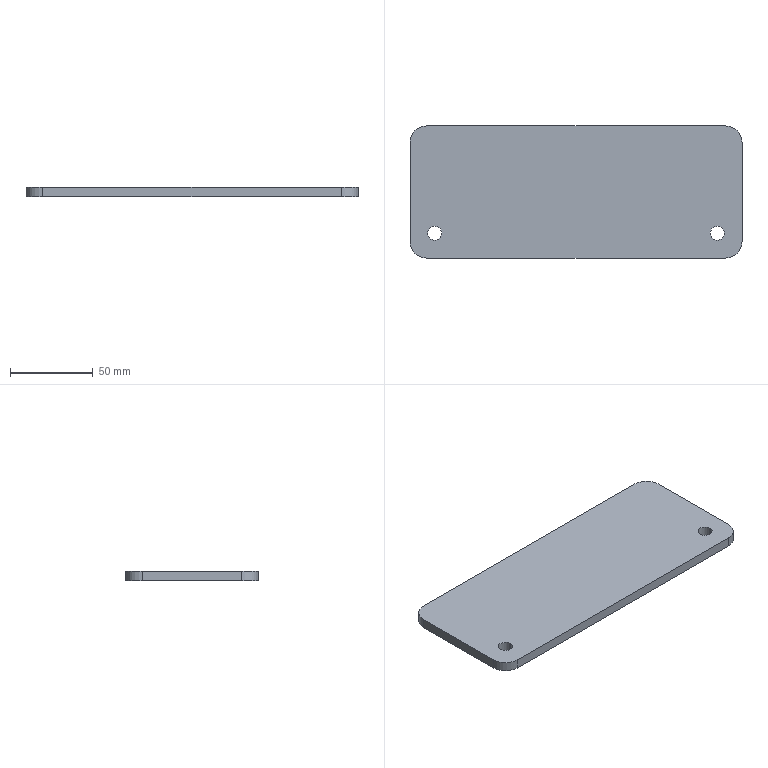Part | SolidWorks | features FlatPattern 1, SMBaseFlange 1, SheetMetal 1 | 1 solid | 14 faces | box 201 x 80 x 6 mm | volume 95284 mm3 | cylinder 8 | plane 6 | commonest cylinder face diameters 8.5 x4 20 x4
STEP:
#1=CARTESIAN_POINT('',(248.25,-78.1,6.));
#2=VERTEX_POINT('',#1);
#3=CARTESIAN_POINT('',(256.75,-78.1,6.));
#4=VERTEX_POINT('',#3);
#5=CARTESIAN_POINT('',(252.5,-78.1,6.));
#6=DIRECTION('',(0.,0.,1.));
#7=DIRECTION('',(1.,0.,0.));
#8=AXIS2_PLACEMENT_3D('',#5,#6,#7);
#9=CIRCLE('',#8,4.25);
#10=EDGE_CURVE('',#2,#4,#9,.T.);
#11=ORIENTED_EDGE('',*,*,#10,.T.);
#12=CARTESIAN_POINT('',(256.75,-78.1,0.));
#13=VERTEX_POINT('',#12);
#14=CARTESIAN_POINT('',(256.75,-78.1,6.));
#15=DIRECTION('',(0.,0.,-1.));
#16=VECTOR('',#15,1000.);
#17=LINE('',#14,#16);
#18=EDGE_CURVE('',#4,#13,#17,.T.);
#19=ORIENTED_EDGE('',*,*,#18,.T.);
#20=CARTESIAN_POINT('',(248.25,-78.1,0.));
#21=VERTEX_POINT('',#20);
#22=CARTESIAN_POINT('',(252.5,-78.1,0.));
#23=DIRECTION('',(0.,0.,1.));
#24=DIRECTION('',(1.,0.,0.));
#25=AXIS2_PLACEMENT_3D('',#22,#23,#24);
#26=CIRCLE('',#25,4.25);
#27=EDGE_CURVE('',#21,#13,#26,.T.);
#28=ORIENTED_EDGE('',*,*,#27,.F.);
#29=CARTESIAN_POINT('',(248.25,-78.1,6.));
#30=DIRECTION('',(0.,0.,-1.));
#31=VECTOR('',#30,1000.);
#32=LINE('',#29,#31);
#33=EDGE_CURVE('',#2,#21,#32,.T.);
#34=ORIENTED_EDGE('',*,*,#33,.F.);
#35=EDGE_LOOP('',(#11,#19,#28,#34));
#36=FACE_OUTER_BOUND('',#35,.T.);
#37=CARTESIAN_POINT('',(252.5,-78.1,6.));
#38=DIRECTION('',(0.,0.,-1.));
#39=DIRECTION('',(-1.,0.,0.));
#40=AXIS2_PLACEMENT_3D('',#37,#38,#39);
#41=CYLINDRICAL_SURFACE('',#40,4.25);
#42=ADVANCED_FACE('',(#36),#41,.F.);
#43=CARTESIAN_POINT('',(419.25,-78.1,6.));
#44=VERTEX_POINT('',#43);
#45=CARTESIAN_POINT('',(427.75,-78.1,6.));
#46=VERTEX_POINT('',#45);
#47=CARTESIAN_POINT('',(423.5,-78.1,6.));
#48=DIRECTION('',(0.,0.,1.));
#49=DIRECTION('',(1.,0.,0.));
#50=AXIS2_PLACEMENT_3D('',#47,#48,#49);
#51=CIRCLE('',#50,4.25);
#52=EDGE_CURVE('',#44,#46,#51,.T.);
#53=ORIENTED_EDGE('',*,*,#52,.T.);
#54=CARTESIAN_POINT('',(427.75,-78.1,0.));
#55=VERTEX_POINT('',#54);
#56=CARTESIAN_POINT('',(427.75,-78.1,6.));
#57=DIRECTION('',(0.,0.,-1.));
#58=VECTOR('',#57,1000.);
#59=LINE('',#56,#58);
#60=EDGE_CURVE('',#46,#55,#59,.T.);
#61=ORIENTED_EDGE('',*,*,#60,.T.);
#62=CARTESIAN_POINT('',(419.25,-78.1,0.));
#63=VERTEX_POINT('',#62);
#64=CARTESIAN_POINT('',(423.5,-78.1,0.));
#65=DIRECTION('',(0.,0.,1.));
#66=DIRECTION('',(1.,0.,0.));
#67=AXIS2_PLACEMENT_3D('',#64,#65,#66);
#68=CIRCLE('',#67,4.25);
#69=EDGE_CURVE('',#63,#55,#68,.T.);
#70=ORIENTED_EDGE('',*,*,#69,.F.);
#71=CARTESIAN_POINT('',(419.25,-78.1,6.));
#72=DIRECTION('',(0.,0.,-1.));
#73=VECTOR('',#72,1000.);
#74=LINE('',#71,#73);
#75=EDGE_CURVE('',#44,#63,#74,.T.);
#76=ORIENTED_EDGE('',*,*,#75,.F.);
#77=EDGE_LOOP('',(#53,#61,#70,#76));
#78=FACE_OUTER_BOUND('',#77,.T.);
#79=CARTESIAN_POINT('',(423.5,-78.1,6.));
#80=DIRECTION('',(0.,0.,-1.));
#81=DIRECTION('',(-1.,0.,0.));
#82=AXIS2_PLACEMENT_3D('',#79,#80,#81);
#83=CYLINDRICAL_SURFACE('',#82,4.25);
#84=ADVANCED_FACE('',(#78),#83,.F.);
#85=ORIENTED_EDGE('',*,*,#52,.F.);
#86=CARTESIAN_POINT('',(423.5,-78.1,6.));
#87=DIRECTION('',(0.,0.,1.));
#88=DIRECTION('',(1.,0.,0.));
#89=AXIS2_PLACEMENT_3D('',#86,#87,#88);
#90=CIRCLE('',#89,4.25);
#91=EDGE_CURVE('',#46,#44,#90,.T.);
#92=ORIENTED_EDGE('',*,*,#91,.F.);
#93=EDGE_LOOP('',(#85,#92));
#94=FACE_BOUND('',#93,.T.);
#95=CARTESIAN_POINT('',(247.5,-13.1,6.));
#96=VERTEX_POINT('',#95);
#97=CARTESIAN_POINT('',(237.5,-23.1,6.));
#98=VERTEX_POINT('',#97);
#99=CARTESIAN_POINT('',(247.5,-23.1,6.));
#100=DIRECTION('',(0.,0.,1.));
#101=DIRECTION('',(1.,0.,0.));
#102=AXIS2_PLACEMENT_3D('',#99,#100,#101);
#103=CIRCLE('',#102,10.);
#104=EDGE_CURVE('',#96,#98,#103,.T.);
#105=ORIENTED_EDGE('',*,*,#104,.T.);
#106=CARTESIAN_POINT('',(237.5,-83.1,6.));
#107=VERTEX_POINT('',#106);
#108=CARTESIAN_POINT('',(237.5,-23.1,6.));
#109=DIRECTION('',(0.,-1.,0.));
#110=VECTOR('',#109,1000.);
#111=LINE('',#108,#110);
#112=EDGE_CURVE('',#98,#107,#111,.T.);
#113=ORIENTED_EDGE('',*,*,#112,.T.);
#114=CARTESIAN_POINT('',(247.5,-93.1,6.));
#115=VERTEX_POINT('',#114);
#116=CARTESIAN_POINT('',(247.5,-83.1,6.));
#117=DIRECTION('',(0.,0.,1.));
#118=DIRECTION('',(-1.,0.,0.));
#119=AXIS2_PLACEMENT_3D('',#116,#117,#118);
#120=CIRCLE('',#119,10.);
#121=EDGE_CURVE('',#107,#115,#120,.T.);
#122=ORIENTED_EDGE('',*,*,#121,.T.);
#123=CARTESIAN_POINT('',(428.5,-93.1,6.));
#124=VERTEX_POINT('',#123);
#125=CARTESIAN_POINT('',(428.5,-93.1,6.));
#126=DIRECTION('',(1.,0.,0.));
#127=VECTOR('',#126,1000.);
#128=LINE('',#125,#127);
#129=EDGE_CURVE('',#115,#124,#128,.T.);
#130=ORIENTED_EDGE('',*,*,#129,.T.);
#131=CARTESIAN_POINT('',(438.5,-83.1,6.));
#132=VERTEX_POINT('',#131);
#133=CARTESIAN_POINT('',(428.5,-83.1,6.));
#134=DIRECTION('',(0.,0.,1.));
#135=DIRECTION('',(-1.,0.,0.));
#136=AXIS2_PLACEMENT_3D('',#133,#134,#135);
#137=CIRCLE('',#136,10.);
#138=EDGE_CURVE('',#124,#132,#137,.T.);
#139=ORIENTED_EDGE('',*,*,#138,.T.);
#140=CARTESIAN_POINT('',(438.5,-23.1,6.));
#141=VERTEX_POINT('',#140);
#142=CARTESIAN_POINT('',(438.5,-23.1,6.));
#143=DIRECTION('',(0.,1.,0.));
#144=VECTOR('',#143,1000.);
#145=LINE('',#142,#144);
#146=EDGE_CURVE('',#132,#141,#145,.T.);
#147=ORIENTED_EDGE('',*,*,#146,.T.);
#148=CARTESIAN_POINT('',(428.5,-13.1,6.));
#149=VERTEX_POINT('',#148);
#150=CARTESIAN_POINT('',(428.5,-23.1,6.));
#151=DIRECTION('',(0.,0.,1.));
#152=DIRECTION('',(-1.,0.,0.));
#153=AXIS2_PLACEMENT_3D('',#150,#151,#152);
#154=CIRCLE('',#153,10.);
#155=EDGE_CURVE('',#141,#149,#154,.T.);
#156=ORIENTED_EDGE('',*,*,#155,.T.);
#157=CARTESIAN_POINT('',(428.5,-13.1,6.));
#158=DIRECTION('',(-1.,0.,0.));
#159=VECTOR('',#158,1000.);
#160=LINE('',#157,#159);
#161=EDGE_CURVE('',#149,#96,#160,.T.);
#162=ORIENTED_EDGE('',*,*,#161,.T.);
#163=EDGE_LOOP('',(#105,#113,#122,#130,#139,#147,#156,#162));
#164=FACE_OUTER_BOUND('',#163,.T.);
#165=ORIENTED_EDGE('',*,*,#10,.F.);
#166=CARTESIAN_POINT('',(252.5,-78.1,6.));
#167=DIRECTION('',(0.,0.,1.));
#168=DIRECTION('',(1.,0.,0.));
#169=AXIS2_PLACEMENT_3D('',#166,#167,#168);
#170=CIRCLE('',#169,4.25);
#171=EDGE_CURVE('',#4,#2,#170,.T.);
#172=ORIENTED_EDGE('',*,*,#171,.F.);
#173=EDGE_LOOP('',(#165,#172));
#174=FACE_BOUND('',#173,.T.);
#175=CARTESIAN_POINT('',(247.5,-23.1,6.));
#176=DIRECTION('',(0.,0.,1.));
#177=DIRECTION('',(1.,0.,0.));
#178=AXIS2_PLACEMENT_3D('',#175,#176,#177);
#179=PLANE('',#178);
#180=ADVANCED_FACE('',(#94,#164,#174),#179,.T.);
#181=CARTESIAN_POINT('',(247.5,-13.1,0.));
#182=VERTEX_POINT('',#181);
#183=CARTESIAN_POINT('',(237.5,-23.1,0.));
#184=VERTEX_POINT('',#183);
#185=CARTESIAN_POINT('',(247.5,-23.1,0.));
#186=DIRECTION('',(0.,0.,1.));
#187=DIRECTION('',(1.,0.,0.));
#188=AXIS2_PLACEMENT_3D('',#185,#186,#187);
#189=CIRCLE('',#188,10.);
#190=EDGE_CURVE('',#182,#184,#189,.T.);
#191=ORIENTED_EDGE('',*,*,#190,.F.);
#192=CARTESIAN_POINT('',(428.5,-13.1,0.));
#193=VERTEX_POINT('',#192);
#194=CARTESIAN_POINT('',(428.5,-13.1,0.));
#195=DIRECTION('',(-1.,0.,0.));
#196=VECTOR('',#195,1000.);
#197=LINE('',#194,#196);
#198=EDGE_CURVE('',#193,#182,#197,.T.);
#199=ORIENTED_EDGE('',*,*,#198,.F.);
#200=CARTESIAN_POINT('',(438.5,-23.1,0.));
#201=VERTEX_POINT('',#200);
#202=CARTESIAN_POINT('',(428.5,-23.1,0.));
#203=DIRECTION('',(0.,0.,1.));
#204=DIRECTION('',(-1.,0.,0.));
#205=AXIS2_PLACEMENT_3D('',#202,#203,#204);
#206=CIRCLE('',#205,10.);
#207=EDGE_CURVE('',#201,#193,#206,.T.);
#208=ORIENTED_EDGE('',*,*,#207,.F.);
#209=CARTESIAN_POINT('',(438.5,-83.1,0.));
#210=VERTEX_POINT('',#209);
#211=CARTESIAN_POINT('',(438.5,-23.1,0.));
#212=DIRECTION('',(0.,1.,0.));
#213=VECTOR('',#212,1000.);
#214=LINE('',#211,#213);
#215=EDGE_CURVE('',#210,#201,#214,.T.);
#216=ORIENTED_EDGE('',*,*,#215,.F.);
#217=CARTESIAN_POINT('',(428.5,-93.1,0.));
#218=VERTEX_POINT('',#217);
#219=CARTESIAN_POINT('',(428.5,-83.1,0.));
#220=DIRECTION('',(0.,0.,1.));
#221=DIRECTION('',(-1.,0.,0.));
#222=AXIS2_PLACEMENT_3D('',#219,#220,#221);
#223=CIRCLE('',#222,10.);
#224=EDGE_CURVE('',#218,#210,#223,.T.);
#225=ORIENTED_EDGE('',*,*,#224,.F.);
#226=CARTESIAN_POINT('',(247.5,-93.1,0.));
#227=VERTEX_POINT('',#226);
#228=CARTESIAN_POINT('',(428.5,-93.1,0.));
#229=DIRECTION('',(1.,0.,0.));
#230=VECTOR('',#229,1000.);
#231=LINE('',#228,#230);
#232=EDGE_CURVE('',#227,#218,#231,.T.);
#233=ORIENTED_EDGE('',*,*,#232,.F.);
#234=CARTESIAN_POINT('',(237.5,-83.1,0.));
#235=VERTEX_POINT('',#234);
#236=CARTESIAN_POINT('',(247.5,-83.1,0.));
#237=DIRECTION('',(0.,0.,1.));
#238=DIRECTION('',(-1.,0.,0.));
#239=AXIS2_PLACEMENT_3D('',#236,#237,#238);
#240=CIRCLE('',#239,10.);
#241=EDGE_CURVE('',#235,#227,#240,.T.);
#242=ORIENTED_EDGE('',*,*,#241,.F.);
#243=CARTESIAN_POINT('',(237.5,-23.1,0.));
#244=DIRECTION('',(0.,-1.,0.));
#245=VECTOR('',#244,1000.);
#246=LINE('',#243,#245);
#247=EDGE_CURVE('',#184,#235,#246,.T.);
#248=ORIENTED_EDGE('',*,*,#247,.F.);
#249=EDGE_LOOP('',(#191,#199,#208,#216,#225,#233,#242,#248));
#250=FACE_OUTER_BOUND('',#249,.T.);
#251=ORIENTED_EDGE('',*,*,#69,.T.);
#252=CARTESIAN_POINT('',(423.5,-78.1,0.));
#253=DIRECTION('',(0.,0.,1.));
#254=DIRECTION('',(1.,0.,0.));
#255=AXIS2_PLACEMENT_3D('',#252,#253,#254);
#256=CIRCLE('',#255,4.25);
#257=EDGE_CURVE('',#55,#63,#256,.T.);
#258=ORIENTED_EDGE('',*,*,#257,.T.);
#259=EDGE_LOOP('',(#251,#258));
#260=FACE_BOUND('',#259,.T.);
#261=ORIENTED_EDGE('',*,*,#27,.T.);
#262=CARTESIAN_POINT('',(252.5,-78.1,0.));
#263=DIRECTION('',(0.,0.,1.));
#264=DIRECTION('',(1.,0.,0.));
#265=AXIS2_PLACEMENT_3D('',#262,#263,#264);
#266=CIRCLE('',#265,4.25);
#267=EDGE_CURVE('',#13,#21,#266,.T.);
#268=ORIENTED_EDGE('',*,*,#267,.T.);
#269=EDGE_LOOP('',(#261,#268));
#270=FACE_BOUND('',#269,.T.);
#271=CARTESIAN_POINT('',(247.5,-23.1,0.));
#272=DIRECTION('',(0.,0.,1.));
#273=DIRECTION('',(1.,0.,0.));
#274=AXIS2_PLACEMENT_3D('',#271,#272,#273);
#275=PLANE('',#274);
#276=ADVANCED_FACE('',(#250,#260,#270),#275,.F.);
#277=ORIENTED_EDGE('',*,*,#190,.T.);
#278=CARTESIAN_POINT('',(237.5,-23.1,6.));
#279=DIRECTION('',(0.,0.,-1.));
#280=VECTOR('',#279,1000.);
#281=LINE('',#278,#280);
#282=EDGE_CURVE('',#98,#184,#281,.T.);
#283=ORIENTED_EDGE('',*,*,#282,.F.);
#284=ORIENTED_EDGE('',*,*,#104,.F.);
#285=CARTESIAN_POINT('',(247.5,-13.1,6.));
#286=DIRECTION('',(0.,0.,-1.));
#287=VECTOR('',#286,1000.);
#288=LINE('',#285,#287);
#289=EDGE_CURVE('',#96,#182,#288,.T.);
#290=ORIENTED_EDGE('',*,*,#289,.T.);
#291=EDGE_LOOP('',(#277,#283,#284,#290));
#292=FACE_OUTER_BOUND('',#291,.T.);
#293=CARTESIAN_POINT('',(247.5,-23.1,6.));
#294=DIRECTION('',(0.,0.,-1.));
#295=DIRECTION('',(-1.,0.,0.));
#296=AXIS2_PLACEMENT_3D('',#293,#294,#295);
#297=CYLINDRICAL_SURFACE('',#296,10.);
#298=ADVANCED_FACE('',(#292),#297,.T.);
#299=ORIENTED_EDGE('',*,*,#247,.T.);
#300=CARTESIAN_POINT('',(237.5,-83.1,6.));
#301=DIRECTION('',(0.,0.,-1.));
#302=VECTOR('',#301,1000.);
#303=LINE('',#300,#302);
#304=EDGE_CURVE('',#107,#235,#303,.T.);
#305=ORIENTED_EDGE('',*,*,#304,.F.);
#306=ORIENTED_EDGE('',*,*,#112,.F.);
#307=ORIENTED_EDGE('',*,*,#282,.T.);
#308=EDGE_LOOP('',(#299,#305,#306,#307));
#309=FACE_OUTER_BOUND('',#308,.T.);
#310=CARTESIAN_POINT('',(237.5,-23.1,6.));
#311=DIRECTION('',(1.,0.,0.));
#312=DIRECTION('',(0.,0.,-1.));
#313=AXIS2_PLACEMENT_3D('',#310,#311,#312);
#314=PLANE('',#313);
#315=ADVANCED_FACE('',(#309),#314,.F.);
#316=ORIENTED_EDGE('',*,*,#241,.T.);
#317=CARTESIAN_POINT('',(247.5,-93.1,6.));
#318=DIRECTION('',(0.,0.,-1.));
#319=VECTOR('',#318,1000.);
#320=LINE('',#317,#319);
#321=EDGE_CURVE('',#115,#227,#320,.T.);
#322=ORIENTED_EDGE('',*,*,#321,.F.);
#323=ORIENTED_EDGE('',*,*,#121,.F.);
#324=ORIENTED_EDGE('',*,*,#304,.T.);
#325=EDGE_LOOP('',(#316,#322,#323,#324));
#326=FACE_OUTER_BOUND('',#325,.T.);
#327=CARTESIAN_POINT('',(247.5,-83.1,6.));
#328=DIRECTION('',(0.,0.,-1.));
#329=DIRECTION('',(-1.,0.,0.));
#330=AXIS2_PLACEMENT_3D('',#327,#328,#329);
#331=CYLINDRICAL_SURFACE('',#330,10.);
#332=ADVANCED_FACE('',(#326),#331,.T.);
#333=ORIENTED_EDGE('',*,*,#232,.T.);
#334=CARTESIAN_POINT('',(428.5,-93.1,6.));
#335=DIRECTION('',(0.,0.,-1.));
#336=VECTOR('',#335,1000.);
#337=LINE('',#334,#336);
#338=EDGE_CURVE('',#124,#218,#337,.T.);
#339=ORIENTED_EDGE('',*,*,#338,.F.);
#340=ORIENTED_EDGE('',*,*,#129,.F.);
#341=ORIENTED_EDGE('',*,*,#321,.T.);
#342=EDGE_LOOP('',(#333,#339,#340,#341));
#343=FACE_OUTER_BOUND('',#342,.T.);
#344=CARTESIAN_POINT('',(428.5,-93.1,6.));
#345=DIRECTION('',(0.,1.,0.));
#346=DIRECTION('',(-1.,0.,0.));
#347=AXIS2_PLACEMENT_3D('',#344,#345,#346);
#348=PLANE('',#347);
#349=ADVANCED_FACE('',(#343),#348,.F.);
#350=ORIENTED_EDGE('',*,*,#224,.T.);
#351=CARTESIAN_POINT('',(438.5,-83.1,6.));
#352=DIRECTION('',(0.,0.,-1.));
#353=VECTOR('',#352,1000.);
#354=LINE('',#351,#353);
#355=EDGE_CURVE('',#132,#210,#354,.T.);
#356=ORIENTED_EDGE('',*,*,#355,.F.);
#357=ORIENTED_EDGE('',*,*,#138,.F.);
#358=ORIENTED_EDGE('',*,*,#338,.T.);
#359=EDGE_LOOP('',(#350,#356,#357,#358));
#360=FACE_OUTER_BOUND('',#359,.T.);
#361=CARTESIAN_POINT('',(428.5,-83.1,6.));
#362=DIRECTION('',(0.,0.,-1.));
#363=DIRECTION('',(-1.,0.,0.));
#364=AXIS2_PLACEMENT_3D('',#361,#362,#363);
#365=CYLINDRICAL_SURFACE('',#364,10.);
#366=ADVANCED_FACE('',(#360),#365,.T.);
#367=ORIENTED_EDGE('',*,*,#215,.T.);
#368=CARTESIAN_POINT('',(438.5,-23.1,6.));
#369=DIRECTION('',(0.,0.,-1.));
#370=VECTOR('',#369,1000.);
#371=LINE('',#368,#370);
#372=EDGE_CURVE('',#141,#201,#371,.T.);
#373=ORIENTED_EDGE('',*,*,#372,.F.);
#374=ORIENTED_EDGE('',*,*,#146,.F.);
#375=ORIENTED_EDGE('',*,*,#355,.T.);
#376=EDGE_LOOP('',(#367,#373,#374,#375));
#377=FACE_OUTER_BOUND('',#376,.T.);
#378=CARTESIAN_POINT('',(438.5,-23.1,6.));
#379=DIRECTION('',(-1.,0.,0.));
#380=DIRECTION('',(0.,0.,1.));
#381=AXIS2_PLACEMENT_3D('',#378,#379,#380);
#382=PLANE('',#381);
#383=ADVANCED_FACE('',(#377),#382,.F.);
#384=ORIENTED_EDGE('',*,*,#207,.T.);
#385=CARTESIAN_POINT('',(428.5,-13.1,6.));
#386=DIRECTION('',(0.,0.,-1.));
#387=VECTOR('',#386,1000.);
#388=LINE('',#385,#387);
#389=EDGE_CURVE('',#149,#193,#388,.T.);
#390=ORIENTED_EDGE('',*,*,#389,.F.);
#391=ORIENTED_EDGE('',*,*,#155,.F.);
#392=ORIENTED_EDGE('',*,*,#372,.T.);
#393=EDGE_LOOP('',(#384,#390,#391,#392));
#394=FACE_OUTER_BOUND('',#393,.T.);
#395=CARTESIAN_POINT('',(428.5,-23.1,6.));
#396=DIRECTION('',(0.,0.,-1.));
#397=DIRECTION('',(-1.,0.,0.));
#398=AXIS2_PLACEMENT_3D('',#395,#396,#397);
#399=CYLINDRICAL_SURFACE('',#398,10.);
#400=ADVANCED_FACE('',(#394),#399,.T.);
#401=ORIENTED_EDGE('',*,*,#198,.T.);
#402=ORIENTED_EDGE('',*,*,#289,.F.);
#403=ORIENTED_EDGE('',*,*,#161,.F.);
#404=ORIENTED_EDGE('',*,*,#389,.T.);
#405=EDGE_LOOP('',(#401,#402,#403,#404));
#406=FACE_OUTER_BOUND('',#405,.T.);
#407=CARTESIAN_POINT('',(428.5,-13.1,6.));
#408=DIRECTION('',(0.,-1.,0.));
#409=DIRECTION('',(1.,0.,0.));
#410=AXIS2_PLACEMENT_3D('',#407,#408,#409);
#411=PLANE('',#410);
#412=ADVANCED_FACE('',(#406),#411,.F.);
#413=ORIENTED_EDGE('',*,*,#60,.F.);
#414=ORIENTED_EDGE('',*,*,#91,.T.);
#415=ORIENTED_EDGE('',*,*,#75,.T.);
#416=ORIENTED_EDGE('',*,*,#257,.F.);
#417=EDGE_LOOP('',(#413,#414,#415,#416));
#418=FACE_OUTER_BOUND('',#417,.T.);
#419=CARTESIAN_POINT('',(423.5,-78.1,6.));
#420=DIRECTION('',(0.,0.,-1.));
#421=DIRECTION('',(-1.,0.,0.));
#422=AXIS2_PLACEMENT_3D('',#419,#420,#421);
#423=CYLINDRICAL_SURFACE('',#422,4.25);
#424=ADVANCED_FACE('',(#418),#423,.F.);
#425=ORIENTED_EDGE('',*,*,#18,.F.);
#426=ORIENTED_EDGE('',*,*,#171,.T.);
#427=ORIENTED_EDGE('',*,*,#33,.T.);
#428=ORIENTED_EDGE('',*,*,#267,.F.);
#429=EDGE_LOOP('',(#425,#426,#427,#428));
#430=FACE_OUTER_BOUND('',#429,.T.);
#431=CARTESIAN_POINT('',(252.5,-78.1,6.));
#432=DIRECTION('',(0.,0.,-1.));
#433=DIRECTION('',(-1.,0.,0.));
#434=AXIS2_PLACEMENT_3D('',#431,#432,#433);
#435=CYLINDRICAL_SURFACE('',#434,4.25);
#436=ADVANCED_FACE('',(#430),#435,.F.);
#437=CLOSED_SHELL('',(#42,#84,#180,#276,#298,#315,#332,#349,#366,#383,#400,#412,#424,#436));
#438=MANIFOLD_SOLID_BREP('',#437);
#439=CARTESIAN_POINT('',(0.,0.,0.));
#440=DIRECTION('',(0.,0.,1.));
#441=DIRECTION('',(1.,0.,0.));
#442=AXIS2_PLACEMENT_3D('',#439,#440,#441);
#443=(LENGTH_UNIT()NAMED_UNIT(*)SI_UNIT(.MILLI.,.METRE.));
#444=UNCERTAINTY_MEASURE_WITH_UNIT(LENGTH_MEASURE(0.00001),#443,'','');
#445=(NAMED_UNIT(*)PLANE_ANGLE_UNIT()SI_UNIT($,.RADIAN.));
#446=(NAMED_UNIT(*)SI_UNIT($,.STERADIAN.)SOLID_ANGLE_UNIT());
#447=(GEOMETRIC_REPRESENTATION_CONTEXT(3)GLOBAL_UNCERTAINTY_ASSIGNED_CONTEXT((#444))GLOBAL_UNIT_ASSIGNED_CONTEXT((#443,#445,#446))REPRESENTATION_CONTEXT('',''));
#448=ADVANCED_BREP_SHAPE_REPRESENTATION('',(#438,#442),#447);